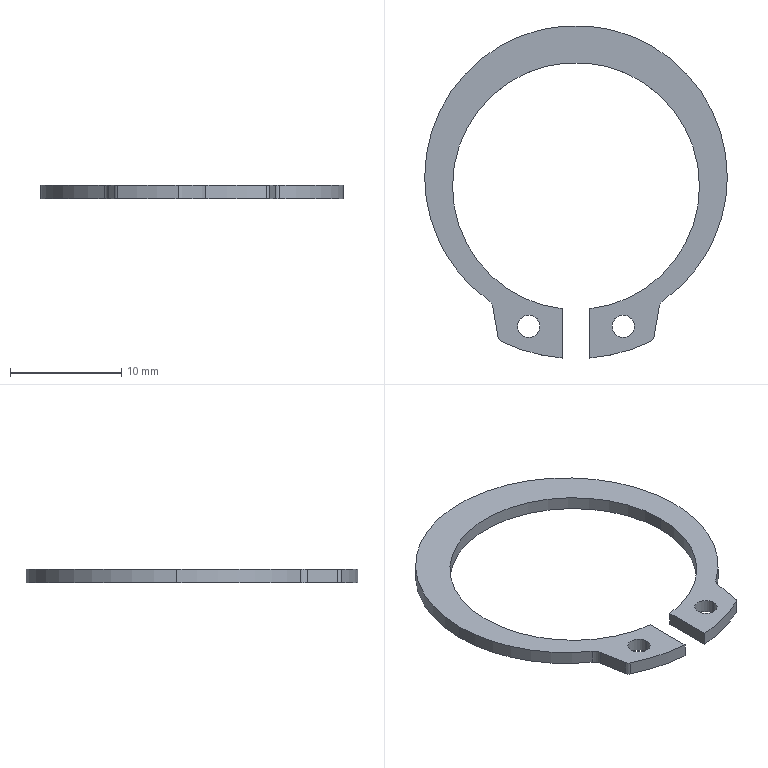Part | SolidWorks | features MoveCopyBody 1, Stock 1 | 1 solid | 22 faces | box 27.2 x 29.88 x 1.2 mm | volume 261.105 mm3 | cylinder 16 | plane 6 | commonest cylinder face diameters 2 x6 22.2 x3 27.2 x3 1 x2 31 x2
STEP:
#1=CARTESIAN_POINT('',(3.25,-12.603,-1.2));
#2=VERTEX_POINT('',#1);
#3=CARTESIAN_POINT('',(5.25,-12.603,-1.2));
#4=VERTEX_POINT('',#3);
#5=CARTESIAN_POINT('',(4.25,-12.603,-1.2));
#6=DIRECTION('',(0.,0.,1.));
#7=DIRECTION('',(-1.,0.,0.));
#8=AXIS2_PLACEMENT_3D('',#5,#6,#7);
#9=CIRCLE('',#8,1.);
#10=EDGE_CURVE('',#2,#4,#9,.T.);
#11=ORIENTED_EDGE('',*,*,#10,.F.);
#12=CARTESIAN_POINT('',(3.25,-12.603,0.));
#13=VERTEX_POINT('',#12);
#14=CARTESIAN_POINT('',(3.25,-12.603,-1.2));
#15=DIRECTION('',(0.,0.,1.));
#16=VECTOR('',#15,1000.);
#17=LINE('',#14,#16);
#18=EDGE_CURVE('',#2,#13,#17,.T.);
#19=ORIENTED_EDGE('',*,*,#18,.T.);
#20=CARTESIAN_POINT('',(5.25,-12.603,0.));
#21=VERTEX_POINT('',#20);
#22=CARTESIAN_POINT('',(4.25,-12.603,0.));
#23=DIRECTION('',(0.,0.,1.));
#24=DIRECTION('',(-1.,0.,0.));
#25=AXIS2_PLACEMENT_3D('',#22,#23,#24);
#26=CIRCLE('',#25,1.);
#27=EDGE_CURVE('',#13,#21,#26,.T.);
#28=ORIENTED_EDGE('',*,*,#27,.T.);
#29=CARTESIAN_POINT('',(5.25,-12.603,-1.2));
#30=DIRECTION('',(0.,0.,1.));
#31=VECTOR('',#30,1000.);
#32=LINE('',#29,#31);
#33=EDGE_CURVE('',#4,#21,#32,.T.);
#34=ORIENTED_EDGE('',*,*,#33,.F.);
#35=EDGE_LOOP('',(#11,#19,#28,#34));
#36=FACE_OUTER_BOUND('',#35,.T.);
#37=CARTESIAN_POINT('',(4.25,-12.603,-1.2));
#38=DIRECTION('',(0.,0.,1.));
#39=DIRECTION('',(1.,0.,0.));
#40=AXIS2_PLACEMENT_3D('',#37,#38,#39);
#41=CYLINDRICAL_SURFACE('',#40,1.);
#42=ADVANCED_FACE('',(#36),#41,.F.);
#43=CARTESIAN_POINT('',(-5.25,-12.603,-1.2));
#44=VERTEX_POINT('',#43);
#45=CARTESIAN_POINT('',(-3.25,-12.603,-1.2));
#46=VERTEX_POINT('',#45);
#47=CARTESIAN_POINT('',(-4.25,-12.603,-1.2));
#48=DIRECTION('',(0.,0.,1.));
#49=DIRECTION('',(1.,0.,0.));
#50=AXIS2_PLACEMENT_3D('',#47,#48,#49);
#51=CIRCLE('',#50,1.);
#52=EDGE_CURVE('',#44,#46,#51,.T.);
#53=ORIENTED_EDGE('',*,*,#52,.F.);
#54=CARTESIAN_POINT('',(-5.25,-12.603,0.));
#55=VERTEX_POINT('',#54);
#56=CARTESIAN_POINT('',(-5.25,-12.603,-1.2));
#57=DIRECTION('',(0.,0.,1.));
#58=VECTOR('',#57,1000.);
#59=LINE('',#56,#58);
#60=EDGE_CURVE('',#44,#55,#59,.T.);
#61=ORIENTED_EDGE('',*,*,#60,.T.);
#62=CARTESIAN_POINT('',(-3.25,-12.603,0.));
#63=VERTEX_POINT('',#62);
#64=CARTESIAN_POINT('',(-4.25,-12.603,0.));
#65=DIRECTION('',(0.,0.,1.));
#66=DIRECTION('',(1.,0.,0.));
#67=AXIS2_PLACEMENT_3D('',#64,#65,#66);
#68=CIRCLE('',#67,1.);
#69=EDGE_CURVE('',#55,#63,#68,.T.);
#70=ORIENTED_EDGE('',*,*,#69,.T.);
#71=CARTESIAN_POINT('',(-3.25,-12.603,-1.2));
#72=DIRECTION('',(0.,0.,1.));
#73=VECTOR('',#72,1000.);
#74=LINE('',#71,#73);
#75=EDGE_CURVE('',#46,#63,#74,.T.);
#76=ORIENTED_EDGE('',*,*,#75,.F.);
#77=EDGE_LOOP('',(#53,#61,#70,#76));
#78=FACE_OUTER_BOUND('',#77,.T.);
#79=CARTESIAN_POINT('',(-4.25,-12.603,-1.2));
#80=DIRECTION('',(0.,0.,1.));
#81=DIRECTION('',(1.,0.,0.));
#82=AXIS2_PLACEMENT_3D('',#79,#80,#81);
#83=CYLINDRICAL_SURFACE('',#82,1.);
#84=ADVANCED_FACE('',(#78),#83,.F.);
#85=CARTESIAN_POINT('',(13.6,0.83,-1.2));
#86=VERTEX_POINT('',#85);
#87=CARTESIAN_POINT('',(-13.6,0.83,-1.2));
#88=VERTEX_POINT('',#87);
#89=CARTESIAN_POINT('',(0.,0.83,-1.2));
#90=DIRECTION('',(0.,0.,1.));
#91=DIRECTION('',(1.,0.,0.));
#92=AXIS2_PLACEMENT_3D('',#89,#90,#91);
#93=CIRCLE('',#92,13.6);
#94=EDGE_CURVE('',#86,#88,#93,.T.);
#95=ORIENTED_EDGE('',*,*,#94,.T.);
#96=CARTESIAN_POINT('',(-13.6,0.83,0.));
#97=VERTEX_POINT('',#96);
#98=CARTESIAN_POINT('',(-13.6,0.83,-1.2));
#99=DIRECTION('',(0.,0.,1.));
#100=VECTOR('',#99,1000.);
#101=LINE('',#98,#100);
#102=EDGE_CURVE('',#88,#97,#101,.T.);
#103=ORIENTED_EDGE('',*,*,#102,.T.);
#104=CARTESIAN_POINT('',(13.6,0.83,0.));
#105=VERTEX_POINT('',#104);
#106=CARTESIAN_POINT('',(0.,0.83,0.));
#107=DIRECTION('',(0.,0.,1.));
#108=DIRECTION('',(1.,0.,0.));
#109=AXIS2_PLACEMENT_3D('',#106,#107,#108);
#110=CIRCLE('',#109,13.6);
#111=EDGE_CURVE('',#105,#97,#110,.T.);
#112=ORIENTED_EDGE('',*,*,#111,.F.);
#113=CARTESIAN_POINT('',(13.6,0.83,-1.2));
#114=DIRECTION('',(0.,0.,1.));
#115=VECTOR('',#114,1000.);
#116=LINE('',#113,#115);
#117=EDGE_CURVE('',#86,#105,#116,.T.);
#118=ORIENTED_EDGE('',*,*,#117,.F.);
#119=EDGE_LOOP('',(#95,#103,#112,#118));
#120=FACE_OUTER_BOUND('',#119,.T.);
#121=CARTESIAN_POINT('',(0.,0.83,-1.2));
#122=DIRECTION('',(0.,0.,1.));
#123=DIRECTION('',(1.,0.,0.));
#124=AXIS2_PLACEMENT_3D('',#121,#122,#123);
#125=CYLINDRICAL_SURFACE('',#124,13.6);
#126=ADVANCED_FACE('',(#120),#125,.T.);
#127=CARTESIAN_POINT('',(7.88,-10.255,-1.2));
#128=VERTEX_POINT('',#127);
#129=CARTESIAN_POINT('',(0.,0.83,-1.2));
#130=DIRECTION('',(0.,0.,1.));
#131=DIRECTION('',(1.,0.,0.));
#132=AXIS2_PLACEMENT_3D('',#129,#130,#131);
#133=CIRCLE('',#132,13.6);
#134=EDGE_CURVE('',#128,#86,#133,.T.);
#135=ORIENTED_EDGE('',*,*,#134,.T.);
#136=ORIENTED_EDGE('',*,*,#117,.T.);
#137=CARTESIAN_POINT('',(7.88,-10.255,0.));
#138=VERTEX_POINT('',#137);
#139=CARTESIAN_POINT('',(0.,0.83,0.));
#140=DIRECTION('',(0.,0.,1.));
#141=DIRECTION('',(1.,0.,0.));
#142=AXIS2_PLACEMENT_3D('',#139,#140,#141);
#143=CIRCLE('',#142,13.6);
#144=EDGE_CURVE('',#138,#105,#143,.T.);
#145=ORIENTED_EDGE('',*,*,#144,.F.);
#146=CARTESIAN_POINT('',(7.88,-10.255,-1.2));
#147=DIRECTION('',(0.,0.,-1.));
#148=VECTOR('',#147,1000.);
#149=LINE('',#146,#148);
#150=EDGE_CURVE('',#138,#128,#149,.T.);
#151=ORIENTED_EDGE('',*,*,#150,.T.);
#152=EDGE_LOOP('',(#135,#136,#145,#151));
#153=FACE_OUTER_BOUND('',#152,.T.);
#154=CARTESIAN_POINT('',(0.,0.83,-1.2));
#155=DIRECTION('',(0.,0.,1.));
#156=DIRECTION('',(1.,0.,0.));
#157=AXIS2_PLACEMENT_3D('',#154,#155,#156);
#158=CYLINDRICAL_SURFACE('',#157,13.6);
#159=ADVANCED_FACE('',(#153),#158,.T.);
#160=CARTESIAN_POINT('',(-1.25,-11.029,-1.2));
#161=VERTEX_POINT('',#160);
#162=CARTESIAN_POINT('',(-11.1,0.,-1.2));
#163=VERTEX_POINT('',#162);
#164=CARTESIAN_POINT('',(0.,0.,-1.2));
#165=DIRECTION('',(0.,0.,-1.));
#166=DIRECTION('',(1.,0.,0.));
#167=AXIS2_PLACEMENT_3D('',#164,#165,#166);
#168=CIRCLE('',#167,11.1);
#169=EDGE_CURVE('',#161,#163,#168,.T.);
#170=ORIENTED_EDGE('',*,*,#169,.T.);
#171=CARTESIAN_POINT('',(-11.1,0.,0.));
#172=VERTEX_POINT('',#171);
#173=CARTESIAN_POINT('',(-11.1,0.,-1.2));
#174=DIRECTION('',(0.,0.,1.));
#175=VECTOR('',#174,1000.);
#176=LINE('',#173,#175);
#177=EDGE_CURVE('',#163,#172,#176,.T.);
#178=ORIENTED_EDGE('',*,*,#177,.T.);
#179=CARTESIAN_POINT('',(-1.25,-11.029,0.));
#180=VERTEX_POINT('',#179);
#181=CARTESIAN_POINT('',(0.,0.,0.));
#182=DIRECTION('',(0.,0.,-1.));
#183=DIRECTION('',(1.,0.,0.));
#184=AXIS2_PLACEMENT_3D('',#181,#182,#183);
#185=CIRCLE('',#184,11.1);
#186=EDGE_CURVE('',#180,#172,#185,.T.);
#187=ORIENTED_EDGE('',*,*,#186,.F.);
#188=CARTESIAN_POINT('',(-1.25,-11.029,-1.2));
#189=DIRECTION('',(0.,0.,1.));
#190=VECTOR('',#189,1000.);
#191=LINE('',#188,#190);
#192=EDGE_CURVE('',#161,#180,#191,.T.);
#193=ORIENTED_EDGE('',*,*,#192,.F.);
#194=EDGE_LOOP('',(#170,#178,#187,#193));
#195=FACE_OUTER_BOUND('',#194,.T.);
#196=CARTESIAN_POINT('',(0.,0.,-1.2));
#197=DIRECTION('',(0.,0.,1.));
#198=DIRECTION('',(1.,0.,0.));
#199=AXIS2_PLACEMENT_3D('',#196,#197,#198);
#200=CYLINDRICAL_SURFACE('',#199,11.1);
#201=ADVANCED_FACE('',(#195),#200,.F.);
#202=ORIENTED_EDGE('',*,*,#177,.F.);
#203=CARTESIAN_POINT('',(11.1,0.,-1.2));
#204=VERTEX_POINT('',#203);
#205=CARTESIAN_POINT('',(0.,0.,-1.2));
#206=DIRECTION('',(0.,0.,-1.));
#207=DIRECTION('',(1.,0.,0.));
#208=AXIS2_PLACEMENT_3D('',#205,#206,#207);
#209=CIRCLE('',#208,11.1);
#210=EDGE_CURVE('',#163,#204,#209,.T.);
#211=ORIENTED_EDGE('',*,*,#210,.T.);
#212=CARTESIAN_POINT('',(11.1,0.,0.));
#213=VERTEX_POINT('',#212);
#214=CARTESIAN_POINT('',(11.1,0.,-1.2));
#215=DIRECTION('',(0.,0.,1.));
#216=VECTOR('',#215,1000.);
#217=LINE('',#214,#216);
#218=EDGE_CURVE('',#204,#213,#217,.T.);
#219=ORIENTED_EDGE('',*,*,#218,.T.);
#220=CARTESIAN_POINT('',(0.,0.,0.));
#221=DIRECTION('',(0.,0.,-1.));
#222=DIRECTION('',(1.,0.,0.));
#223=AXIS2_PLACEMENT_3D('',#220,#221,#222);
#224=CIRCLE('',#223,11.1);
#225=EDGE_CURVE('',#172,#213,#224,.T.);
#226=ORIENTED_EDGE('',*,*,#225,.F.);
#227=EDGE_LOOP('',(#202,#211,#219,#226));
#228=FACE_OUTER_BOUND('',#227,.T.);
#229=CARTESIAN_POINT('',(0.,0.,-1.2));
#230=DIRECTION('',(0.,0.,1.));
#231=DIRECTION('',(1.,0.,0.));
#232=AXIS2_PLACEMENT_3D('',#229,#230,#231);
#233=CYLINDRICAL_SURFACE('',#232,11.1);
#234=ADVANCED_FACE('',(#228),#233,.F.);
#235=CARTESIAN_POINT('',(1.25,-15.45,-1.2));
#236=VERTEX_POINT('',#235);
#237=CARTESIAN_POINT('',(6.721,-13.967,-1.2));
#238=VERTEX_POINT('',#237);
#239=CARTESIAN_POINT('',(0.,0.,-1.2));
#240=DIRECTION('',(0.,0.,1.));
#241=DIRECTION('',(-1.,0.,0.));
#242=AXIS2_PLACEMENT_3D('',#239,#240,#241);
#243=CIRCLE('',#242,15.5);
#244=EDGE_CURVE('',#236,#238,#243,.T.);
#245=ORIENTED_EDGE('',*,*,#244,.T.);
#246=CARTESIAN_POINT('',(6.721,-13.967,0.));
#247=VERTEX_POINT('',#246);
#248=CARTESIAN_POINT('',(6.721,-13.967,-1.2));
#249=DIRECTION('',(0.,0.,1.));
#250=VECTOR('',#249,1000.);
#251=LINE('',#248,#250);
#252=EDGE_CURVE('',#238,#247,#251,.T.);
#253=ORIENTED_EDGE('',*,*,#252,.T.);
#254=CARTESIAN_POINT('',(1.25,-15.45,0.));
#255=VERTEX_POINT('',#254);
#256=CARTESIAN_POINT('',(0.,0.,0.));
#257=DIRECTION('',(0.,0.,1.));
#258=DIRECTION('',(-1.,0.,0.));
#259=AXIS2_PLACEMENT_3D('',#256,#257,#258);
#260=CIRCLE('',#259,15.5);
#261=EDGE_CURVE('',#255,#247,#260,.T.);
#262=ORIENTED_EDGE('',*,*,#261,.F.);
#263=CARTESIAN_POINT('',(1.25,-15.45,-1.2));
#264=DIRECTION('',(0.,0.,1.));
#265=VECTOR('',#264,1000.);
#266=LINE('',#263,#265);
#267=EDGE_CURVE('',#236,#255,#266,.T.);
#268=ORIENTED_EDGE('',*,*,#267,.F.);
#269=EDGE_LOOP('',(#245,#253,#262,#268));
#270=FACE_OUTER_BOUND('',#269,.T.);
#271=CARTESIAN_POINT('',(0.,0.,-1.2));
#272=DIRECTION('',(0.,0.,1.));
#273=DIRECTION('',(1.,0.,0.));
#274=AXIS2_PLACEMENT_3D('',#271,#272,#273);
#275=CYLINDRICAL_SURFACE('',#274,15.5);
#276=ADVANCED_FACE('',(#270),#275,.T.);
#277=CARTESIAN_POINT('',(1.25,-11.029,0.));
#278=VERTEX_POINT('',#277);
#279=CARTESIAN_POINT('',(1.25,-11.029,0.));
#280=DIRECTION('',(0.,-1.,0.));
#281=VECTOR('',#280,1000.);
#282=LINE('',#279,#281);
#283=EDGE_CURVE('',#278,#255,#282,.T.);
#284=ORIENTED_EDGE('',*,*,#283,.F.);
#285=CARTESIAN_POINT('',(1.25,-11.029,-1.2));
#286=VERTEX_POINT('',#285);
#287=CARTESIAN_POINT('',(1.25,-11.029,-1.2));
#288=DIRECTION('',(0.,0.,1.));
#289=VECTOR('',#288,1000.);
#290=LINE('',#287,#289);
#291=EDGE_CURVE('',#286,#278,#290,.T.);
#292=ORIENTED_EDGE('',*,*,#291,.F.);
#293=CARTESIAN_POINT('',(1.25,-11.029,-1.2));
#294=DIRECTION('',(0.,-1.,0.));
#295=VECTOR('',#294,1000.);
#296=LINE('',#293,#295);
#297=EDGE_CURVE('',#286,#236,#296,.T.);
#298=ORIENTED_EDGE('',*,*,#297,.T.);
#299=ORIENTED_EDGE('',*,*,#267,.T.);
#300=EDGE_LOOP('',(#284,#292,#298,#299));
#301=FACE_OUTER_BOUND('',#300,.T.);
#302=CARTESIAN_POINT('',(1.25,-11.029,-1.2));
#303=DIRECTION('',(-1.,0.,0.));
#304=DIRECTION('',(0.,-1.,0.));
#305=AXIS2_PLACEMENT_3D('',#302,#303,#304);
#306=PLANE('',#305);
#307=ADVANCED_FACE('',(#301),#306,.T.);
#308=ORIENTED_EDGE('',*,*,#218,.F.);
#309=CARTESIAN_POINT('',(0.,0.,-1.2));
#310=DIRECTION('',(0.,0.,-1.));
#311=DIRECTION('',(1.,0.,0.));
#312=AXIS2_PLACEMENT_3D('',#309,#310,#311);
#313=CIRCLE('',#312,11.1);
#314=EDGE_CURVE('',#204,#286,#313,.T.);
#315=ORIENTED_EDGE('',*,*,#314,.T.);
#316=ORIENTED_EDGE('',*,*,#291,.T.);
#317=CARTESIAN_POINT('',(0.,0.,0.));
#318=DIRECTION('',(0.,0.,-1.));
#319=DIRECTION('',(1.,0.,0.));
#320=AXIS2_PLACEMENT_3D('',#317,#318,#319);
#321=CIRCLE('',#320,11.1);
#322=EDGE_CURVE('',#213,#278,#321,.T.);
#323=ORIENTED_EDGE('',*,*,#322,.F.);
#324=EDGE_LOOP('',(#308,#315,#316,#323));
#325=FACE_OUTER_BOUND('',#324,.T.);
#326=CARTESIAN_POINT('',(0.,0.,-1.2));
#327=DIRECTION('',(0.,0.,1.));
#328=DIRECTION('',(1.,0.,0.));
#329=AXIS2_PLACEMENT_3D('',#326,#327,#328);
#330=CYLINDRICAL_SURFACE('',#329,11.1);
#331=ADVANCED_FACE('',(#325),#330,.F.);
#332=CARTESIAN_POINT('',(-1.25,-15.45,0.));
#333=VERTEX_POINT('',#332);
#334=CARTESIAN_POINT('',(-1.25,-11.029,0.));
#335=DIRECTION('',(0.,1.,0.));
#336=VECTOR('',#335,1000.);
#337=LINE('',#334,#336);
#338=EDGE_CURVE('',#333,#180,#337,.T.);
#339=ORIENTED_EDGE('',*,*,#338,.F.);
#340=CARTESIAN_POINT('',(-1.25,-15.45,-1.2));
#341=VERTEX_POINT('',#340);
#342=CARTESIAN_POINT('',(-1.25,-15.45,-1.2));
#343=DIRECTION('',(0.,0.,1.));
#344=VECTOR('',#343,1000.);
#345=LINE('',#342,#344);
#346=EDGE_CURVE('',#341,#333,#345,.T.);
#347=ORIENTED_EDGE('',*,*,#346,.F.);
#348=CARTESIAN_POINT('',(-1.25,-11.029,-1.2));
#349=DIRECTION('',(0.,1.,0.));
#350=VECTOR('',#349,1000.);
#351=LINE('',#348,#350);
#352=EDGE_CURVE('',#341,#161,#351,.T.);
#353=ORIENTED_EDGE('',*,*,#352,.T.);
#354=ORIENTED_EDGE('',*,*,#192,.T.);
#355=EDGE_LOOP('',(#339,#347,#353,#354));
#356=FACE_OUTER_BOUND('',#355,.T.);
#357=CARTESIAN_POINT('',(-1.25,-11.029,-1.2));
#358=DIRECTION('',(1.,0.,0.));
#359=DIRECTION('',(0.,1.,0.));
#360=AXIS2_PLACEMENT_3D('',#357,#358,#359);
#361=PLANE('',#360);
#362=ADVANCED_FACE('',(#356),#361,.T.);
#363=CARTESIAN_POINT('',(-6.721,-13.967,0.));
#364=VERTEX_POINT('',#363);
#365=CARTESIAN_POINT('',(0.,0.,0.));
#366=DIRECTION('',(0.,0.,1.));
#367=DIRECTION('',(1.,0.,0.));
#368=AXIS2_PLACEMENT_3D('',#365,#366,#367);
#369=CIRCLE('',#368,15.5);
#370=EDGE_CURVE('',#364,#333,#369,.T.);
#371=ORIENTED_EDGE('',*,*,#370,.F.);
#372=CARTESIAN_POINT('',(-6.721,-13.967,-1.2));
#373=VERTEX_POINT('',#372);
#374=CARTESIAN_POINT('',(-6.721,-13.967,-1.2));
#375=DIRECTION('',(0.,0.,-1.));
#376=VECTOR('',#375,1000.);
#377=LINE('',#374,#376);
#378=EDGE_CURVE('',#364,#373,#377,.T.);
#379=ORIENTED_EDGE('',*,*,#378,.T.);
#380=CARTESIAN_POINT('',(0.,0.,-1.2));
#381=DIRECTION('',(0.,0.,1.));
#382=DIRECTION('',(1.,0.,0.));
#383=AXIS2_PLACEMENT_3D('',#380,#381,#382);
#384=CIRCLE('',#383,15.5);
#385=EDGE_CURVE('',#373,#341,#384,.T.);
#386=ORIENTED_EDGE('',*,*,#385,.T.);
#387=ORIENTED_EDGE('',*,*,#346,.T.);
#388=EDGE_LOOP('',(#371,#379,#386,#387));
#389=FACE_OUTER_BOUND('',#388,.T.);
#390=CARTESIAN_POINT('',(0.,0.,-1.2));
#391=DIRECTION('',(0.,0.,1.));
#392=DIRECTION('',(1.,0.,0.));
#393=AXIS2_PLACEMENT_3D('',#390,#391,#392);
#394=CYLINDRICAL_SURFACE('',#393,15.5);
#395=ADVANCED_FACE('',(#389),#394,.T.);
#396=CARTESIAN_POINT('',(-7.474,-10.896,0.));
#397=VERTEX_POINT('',#396);
#398=CARTESIAN_POINT('',(-6.997,-13.603,0.));
#399=VERTEX_POINT('',#398);
#400=CARTESIAN_POINT('',(-7.547,-10.484,0.));
#401=DIRECTION('',(0.1736,-0.9848,0.));
#402=VECTOR('',#401,1000.);
#403=LINE('',#400,#402);
#404=EDGE_CURVE('',#397,#399,#403,.T.);
#405=ORIENTED_EDGE('',*,*,#404,.F.);
#406=CARTESIAN_POINT('',(-7.474,-10.896,-1.2));
#407=VERTEX_POINT('',#406);
#408=CARTESIAN_POINT('',(-7.474,-10.896,-1.2));
#409=DIRECTION('',(0.,0.,-1.));
#410=VECTOR('',#409,1000.);
#411=LINE('',#408,#410);
#412=EDGE_CURVE('',#397,#407,#411,.T.);
#413=ORIENTED_EDGE('',*,*,#412,.T.);
#414=CARTESIAN_POINT('',(-6.997,-13.603,-1.2));
#415=VERTEX_POINT('',#414);
#416=CARTESIAN_POINT('',(-7.547,-10.484,-1.2));
#417=DIRECTION('',(0.1736,-0.9848,0.));
#418=VECTOR('',#417,1000.);
#419=LINE('',#416,#418);
#420=EDGE_CURVE('',#407,#415,#419,.T.);
#421=ORIENTED_EDGE('',*,*,#420,.T.);
#422=CARTESIAN_POINT('',(-6.997,-13.603,-1.2));
#423=DIRECTION('',(0.,0.,1.));
#424=VECTOR('',#423,1000.);
#425=LINE('',#422,#424);
#426=EDGE_CURVE('',#415,#399,#425,.T.);
#427=ORIENTED_EDGE('',*,*,#426,.T.);
#428=EDGE_LOOP('',(#405,#413,#421,#427));
#429=FACE_OUTER_BOUND('',#428,.T.);
#430=CARTESIAN_POINT('',(-7.547,-10.484,-1.2));
#431=DIRECTION('',(-0.9848,-0.1736,0.));
#432=DIRECTION('',(0.1736,-0.9848,0.));
#433=AXIS2_PLACEMENT_3D('',#430,#431,#432);
#434=PLANE('',#433);
#435=ADVANCED_FACE('',(#429),#434,.T.);
#436=ORIENTED_EDGE('',*,*,#102,.F.);
#437=CARTESIAN_POINT('',(-7.88,-10.255,-1.2));
#438=VERTEX_POINT('',#437);
#439=CARTESIAN_POINT('',(0.,0.83,-1.2));
#440=DIRECTION('',(0.,0.,1.));
#441=DIRECTION('',(1.,0.,0.));
#442=AXIS2_PLACEMENT_3D('',#439,#440,#441);
#443=CIRCLE('',#442,13.6);
#444=EDGE_CURVE('',#88,#438,#443,.T.);
#445=ORIENTED_EDGE('',*,*,#444,.T.);
#446=CARTESIAN_POINT('',(-7.88,-10.255,0.));
#447=VERTEX_POINT('',#446);
#448=CARTESIAN_POINT('',(-7.88,-10.255,-1.2));
#449=DIRECTION('',(0.,0.,1.));
#450=VECTOR('',#449,1000.);
#451=LINE('',#448,#450);
#452=EDGE_CURVE('',#438,#447,#451,.T.);
#453=ORIENTED_EDGE('',*,*,#452,.T.);
#454=CARTESIAN_POINT('',(0.,0.83,0.));
#455=DIRECTION('',(0.,0.,1.));
#456=DIRECTION('',(1.,0.,0.));
#457=AXIS2_PLACEMENT_3D('',#454,#455,#456);
#458=CIRCLE('',#457,13.6);
#459=EDGE_CURVE('',#97,#447,#458,.T.);
#460=ORIENTED_EDGE('',*,*,#459,.F.);
#461=EDGE_LOOP('',(#436,#445,#453,#460));
#462=FACE_OUTER_BOUND('',#461,.T.);
#463=CARTESIAN_POINT('',(0.,0.83,-1.2));
#464=DIRECTION('',(0.,0.,1.));
#465=DIRECTION('',(1.,0.,0.));
#466=AXIS2_PLACEMENT_3D('',#463,#464,#465);
#467=CYLINDRICAL_SURFACE('',#466,13.6);
#468=ADVANCED_FACE('',(#462),#467,.T.);
#469=CARTESIAN_POINT('',(6.997,-13.603,-1.2));
#470=VERTEX_POINT('',#469);
#471=CARTESIAN_POINT('',(7.474,-10.896,-1.2));
#472=VERTEX_POINT('',#471);
#473=CARTESIAN_POINT('',(7.547,-10.484,-1.2));
#474=DIRECTION('',(0.1736,0.9848,0.));
#475=VECTOR('',#474,1000.);
#476=LINE('',#473,#475);
#477=EDGE_CURVE('',#470,#472,#476,.T.);
#478=ORIENTED_EDGE('',*,*,#477,.T.);
#479=CARTESIAN_POINT('',(7.474,-10.896,0.));
#480=VERTEX_POINT('',#479);
#481=CARTESIAN_POINT('',(7.474,-10.896,0.));
#482=DIRECTION('',(0.,0.,1.));
#483=VECTOR('',#482,1000.);
#484=LINE('',#481,#483);
#485=EDGE_CURVE('',#472,#480,#484,.T.);
#486=ORIENTED_EDGE('',*,*,#485,.T.);
#487=CARTESIAN_POINT('',(6.997,-13.603,0.));
#488=VERTEX_POINT('',#487);
#489=CARTESIAN_POINT('',(7.547,-10.484,0.));
#490=DIRECTION('',(0.1736,0.9848,0.));
#491=VECTOR('',#490,1000.);
#492=LINE('',#489,#491);
#493=EDGE_CURVE('',#488,#480,#492,.T.);
#494=ORIENTED_EDGE('',*,*,#493,.F.);
#495=CARTESIAN_POINT('',(6.997,-13.603,-1.2));
#496=DIRECTION('',(0.,0.,-1.));
#497=VECTOR('',#496,1000.);
#498=LINE('',#495,#497);
#499=EDGE_CURVE('',#488,#470,#498,.T.);
#500=ORIENTED_EDGE('',*,*,#499,.T.);
#501=EDGE_LOOP('',(#478,#486,#494,#500));
#502=FACE_OUTER_BOUND('',#501,.T.);
#503=CARTESIAN_POINT('',(7.547,-10.484,-1.2));
#504=DIRECTION('',(0.9848,-0.1736,0.));
#505=DIRECTION('',(0.1736,0.9848,0.));
#506=AXIS2_PLACEMENT_3D('',#503,#504,#505);
#507=PLANE('',#506);
#508=ADVANCED_FACE('',(#502),#507,.T.);
#509=CARTESIAN_POINT('',(4.25,-12.603,-1.2));
#510=DIRECTION('',(0.,0.,1.));
#511=DIRECTION('',(-1.,0.,0.));
#512=AXIS2_PLACEMENT_3D('',#509,#510,#511);
#513=CIRCLE('',#512,1.);
#514=EDGE_CURVE('',#4,#2,#513,.T.);
#515=ORIENTED_EDGE('',*,*,#514,.T.);
#516=ORIENTED_EDGE('',*,*,#10,.T.);
#517=EDGE_LOOP('',(#515,#516));
#518=FACE_BOUND('',#517,.T.);
#519=CARTESIAN_POINT('',(-4.25,-12.603,-1.2));
#520=DIRECTION('',(0.,0.,1.));
#521=DIRECTION('',(1.,0.,0.));
#522=AXIS2_PLACEMENT_3D('',#519,#520,#521);
#523=CIRCLE('',#522,1.);
#524=EDGE_CURVE('',#46,#44,#523,.T.);
#525=ORIENTED_EDGE('',*,*,#524,.T.);
#526=ORIENTED_EDGE('',*,*,#52,.T.);
#527=EDGE_LOOP('',(#525,#526));
#528=FACE_BOUND('',#527,.T.);
#529=ORIENTED_EDGE('',*,*,#385,.F.);
#530=CARTESIAN_POINT('',(-6.505,-13.516,-1.2));
#531=DIRECTION('',(0.,0.,-1.));
#532=DIRECTION('',(-1.,0.,0.));
#533=AXIS2_PLACEMENT_3D('',#530,#531,#532);
#534=CIRCLE('',#533,0.5);
#535=EDGE_CURVE('',#373,#415,#534,.T.);
#536=ORIENTED_EDGE('',*,*,#535,.T.);
#537=ORIENTED_EDGE('',*,*,#420,.F.);
#538=CARTESIAN_POINT('',(-8.459,-11.07,-1.2));
#539=DIRECTION('',(0.,0.,1.));
#540=DIRECTION('',(-1.,0.,0.));
#541=AXIS2_PLACEMENT_3D('',#538,#539,#540);
#542=CIRCLE('',#541,1.);
#543=EDGE_CURVE('',#407,#438,#542,.T.);
#544=ORIENTED_EDGE('',*,*,#543,.T.);
#545=ORIENTED_EDGE('',*,*,#444,.F.);
#546=ORIENTED_EDGE('',*,*,#94,.F.);
#547=ORIENTED_EDGE('',*,*,#134,.F.);
#548=CARTESIAN_POINT('',(8.459,-11.07,-1.2));
#549=DIRECTION('',(0.,0.,1.));
#550=DIRECTION('',(-1.,0.,0.));
#551=AXIS2_PLACEMENT_3D('',#548,#549,#550);
#552=CIRCLE('',#551,1.);
#553=EDGE_CURVE('',#128,#472,#552,.T.);
#554=ORIENTED_EDGE('',*,*,#553,.T.);
#555=ORIENTED_EDGE('',*,*,#477,.F.);
#556=CARTESIAN_POINT('',(6.505,-13.516,-1.2));
#557=DIRECTION('',(0.,0.,-1.));
#558=DIRECTION('',(-1.,0.,0.));
#559=AXIS2_PLACEMENT_3D('',#556,#557,#558);
#560=CIRCLE('',#559,0.5);
#561=EDGE_CURVE('',#470,#238,#560,.T.);
#562=ORIENTED_EDGE('',*,*,#561,.T.);
#563=ORIENTED_EDGE('',*,*,#244,.F.);
#564=ORIENTED_EDGE('',*,*,#297,.F.);
#565=ORIENTED_EDGE('',*,*,#314,.F.);
#566=ORIENTED_EDGE('',*,*,#210,.F.);
#567=ORIENTED_EDGE('',*,*,#169,.F.);
#568=ORIENTED_EDGE('',*,*,#352,.F.);
#569=EDGE_LOOP('',(#529,#536,#537,#544,#545,#546,#547,#554,#555,#562,#563,#564,#565,#566,#567,#568));
#570=FACE_OUTER_BOUND('',#569,.T.);
#571=CARTESIAN_POINT('',(0.,0.,-1.2));
#572=DIRECTION('',(0.,0.,-1.));
#573=DIRECTION('',(-1.,0.,0.));
#574=AXIS2_PLACEMENT_3D('',#571,#572,#573);
#575=PLANE('',#574);
#576=ADVANCED_FACE('',(#518,#528,#570),#575,.T.);
#577=CARTESIAN_POINT('',(4.25,-12.603,0.));
#578=DIRECTION('',(0.,0.,1.));
#579=DIRECTION('',(-1.,0.,0.));
#580=AXIS2_PLACEMENT_3D('',#577,#578,#579);
#581=CIRCLE('',#580,1.);
#582=EDGE_CURVE('',#21,#13,#581,.T.);
#583=ORIENTED_EDGE('',*,*,#582,.F.);
#584=ORIENTED_EDGE('',*,*,#27,.F.);
#585=EDGE_LOOP('',(#583,#584));
#586=FACE_BOUND('',#585,.T.);
#587=CARTESIAN_POINT('',(-4.25,-12.603,0.));
#588=DIRECTION('',(0.,0.,1.));
#589=DIRECTION('',(1.,0.,0.));
#590=AXIS2_PLACEMENT_3D('',#587,#588,#589);
#591=CIRCLE('',#590,1.);
#592=EDGE_CURVE('',#63,#55,#591,.T.);
#593=ORIENTED_EDGE('',*,*,#592,.F.);
#594=ORIENTED_EDGE('',*,*,#69,.F.);
#595=EDGE_LOOP('',(#593,#594));
#596=FACE_BOUND('',#595,.T.);
#597=ORIENTED_EDGE('',*,*,#144,.T.);
#598=ORIENTED_EDGE('',*,*,#111,.T.);
#599=ORIENTED_EDGE('',*,*,#459,.T.);
#600=CARTESIAN_POINT('',(-8.459,-11.07,0.));
#601=DIRECTION('',(0.,0.,-1.));
#602=DIRECTION('',(-1.,0.,0.));
#603=AXIS2_PLACEMENT_3D('',#600,#601,#602);
#604=CIRCLE('',#603,1.);
#605=EDGE_CURVE('',#447,#397,#604,.T.);
#606=ORIENTED_EDGE('',*,*,#605,.T.);
#607=ORIENTED_EDGE('',*,*,#404,.T.);
#608=CARTESIAN_POINT('',(-6.505,-13.516,0.));
#609=DIRECTION('',(0.,0.,1.));
#610=DIRECTION('',(-1.,0.,0.));
#611=AXIS2_PLACEMENT_3D('',#608,#609,#610);
#612=CIRCLE('',#611,0.5);
#613=EDGE_CURVE('',#399,#364,#612,.T.);
#614=ORIENTED_EDGE('',*,*,#613,.T.);
#615=ORIENTED_EDGE('',*,*,#370,.T.);
#616=ORIENTED_EDGE('',*,*,#338,.T.);
#617=ORIENTED_EDGE('',*,*,#186,.T.);
#618=ORIENTED_EDGE('',*,*,#225,.T.);
#619=ORIENTED_EDGE('',*,*,#322,.T.);
#620=ORIENTED_EDGE('',*,*,#283,.T.);
#621=ORIENTED_EDGE('',*,*,#261,.T.);
#622=CARTESIAN_POINT('',(6.505,-13.516,0.));
#623=DIRECTION('',(0.,0.,1.));
#624=DIRECTION('',(-1.,0.,0.));
#625=AXIS2_PLACEMENT_3D('',#622,#623,#624);
#626=CIRCLE('',#625,0.5);
#627=EDGE_CURVE('',#247,#488,#626,.T.);
#628=ORIENTED_EDGE('',*,*,#627,.T.);
#629=ORIENTED_EDGE('',*,*,#493,.T.);
#630=CARTESIAN_POINT('',(8.459,-11.07,0.));
#631=DIRECTION('',(0.,0.,-1.));
#632=DIRECTION('',(-1.,0.,0.));
#633=AXIS2_PLACEMENT_3D('',#630,#631,#632);
#634=CIRCLE('',#633,1.);
#635=EDGE_CURVE('',#480,#138,#634,.T.);
#636=ORIENTED_EDGE('',*,*,#635,.T.);
#637=EDGE_LOOP('',(#597,#598,#599,#606,#607,#614,#615,#616,#617,#618,#619,#620,#621,#628,#629,#636));
#638=FACE_OUTER_BOUND('',#637,.T.);
#639=CARTESIAN_POINT('',(0.,0.,0.));
#640=DIRECTION('',(0.,0.,-1.));
#641=DIRECTION('',(-1.,0.,0.));
#642=AXIS2_PLACEMENT_3D('',#639,#640,#641);
#643=PLANE('',#642);
#644=ADVANCED_FACE('',(#586,#596,#638),#643,.F.);
#645=ORIENTED_EDGE('',*,*,#60,.F.);
#646=ORIENTED_EDGE('',*,*,#524,.F.);
#647=ORIENTED_EDGE('',*,*,#75,.T.);
#648=ORIENTED_EDGE('',*,*,#592,.T.);
#649=EDGE_LOOP('',(#645,#646,#647,#648));
#650=FACE_OUTER_BOUND('',#649,.T.);
#651=CARTESIAN_POINT('',(-4.25,-12.603,-1.2));
#652=DIRECTION('',(0.,0.,1.));
#653=DIRECTION('',(1.,0.,0.));
#654=AXIS2_PLACEMENT_3D('',#651,#652,#653);
#655=CYLINDRICAL_SURFACE('',#654,1.);
#656=ADVANCED_FACE('',(#650),#655,.F.);
#657=ORIENTED_EDGE('',*,*,#18,.F.);
#658=ORIENTED_EDGE('',*,*,#514,.F.);
#659=ORIENTED_EDGE('',*,*,#33,.T.);
#660=ORIENTED_EDGE('',*,*,#582,.T.);
#661=EDGE_LOOP('',(#657,#658,#659,#660));
#662=FACE_OUTER_BOUND('',#661,.T.);
#663=CARTESIAN_POINT('',(4.25,-12.603,-1.2));
#664=DIRECTION('',(0.,0.,1.));
#665=DIRECTION('',(1.,0.,0.));
#666=AXIS2_PLACEMENT_3D('',#663,#664,#665);
#667=CYLINDRICAL_SURFACE('',#666,1.);
#668=ADVANCED_FACE('',(#662),#667,.F.);
#669=ORIENTED_EDGE('',*,*,#535,.F.);
#670=ORIENTED_EDGE('',*,*,#378,.F.);
#671=ORIENTED_EDGE('',*,*,#613,.F.);
#672=ORIENTED_EDGE('',*,*,#426,.F.);
#673=EDGE_LOOP('',(#669,#670,#671,#672));
#674=FACE_OUTER_BOUND('',#673,.T.);
#675=CARTESIAN_POINT('',(-6.505,-13.516,-1.2));
#676=DIRECTION('',(0.,0.,1.));
#677=DIRECTION('',(1.,0.,0.));
#678=AXIS2_PLACEMENT_3D('',#675,#676,#677);
#679=CYLINDRICAL_SURFACE('',#678,0.5);
#680=ADVANCED_FACE('',(#674),#679,.T.);
#681=ORIENTED_EDGE('',*,*,#561,.F.);
#682=ORIENTED_EDGE('',*,*,#499,.F.);
#683=ORIENTED_EDGE('',*,*,#627,.F.);
#684=ORIENTED_EDGE('',*,*,#252,.F.);
#685=EDGE_LOOP('',(#681,#682,#683,#684));
#686=FACE_OUTER_BOUND('',#685,.T.);
#687=CARTESIAN_POINT('',(6.505,-13.516,-1.2));
#688=DIRECTION('',(0.,0.,1.));
#689=DIRECTION('',(1.,0.,0.));
#690=AXIS2_PLACEMENT_3D('',#687,#688,#689);
#691=CYLINDRICAL_SURFACE('',#690,0.5);
#692=ADVANCED_FACE('',(#686),#691,.T.);
#693=ORIENTED_EDGE('',*,*,#553,.F.);
#694=ORIENTED_EDGE('',*,*,#150,.F.);
#695=ORIENTED_EDGE('',*,*,#635,.F.);
#696=ORIENTED_EDGE('',*,*,#485,.F.);
#697=EDGE_LOOP('',(#693,#694,#695,#696));
#698=FACE_OUTER_BOUND('',#697,.T.);
#699=CARTESIAN_POINT('',(8.459,-11.07,-1.2));
#700=DIRECTION('',(0.,0.,1.));
#701=DIRECTION('',(1.,0.,0.));
#702=AXIS2_PLACEMENT_3D('',#699,#700,#701);
#703=CYLINDRICAL_SURFACE('',#702,1.);
#704=ADVANCED_FACE('',(#698),#703,.F.);
#705=ORIENTED_EDGE('',*,*,#543,.F.);
#706=ORIENTED_EDGE('',*,*,#412,.F.);
#707=ORIENTED_EDGE('',*,*,#605,.F.);
#708=ORIENTED_EDGE('',*,*,#452,.F.);
#709=EDGE_LOOP('',(#705,#706,#707,#708));
#710=FACE_OUTER_BOUND('',#709,.T.);
#711=CARTESIAN_POINT('',(-8.459,-11.07,-1.2));
#712=DIRECTION('',(0.,0.,1.));
#713=DIRECTION('',(1.,0.,0.));
#714=AXIS2_PLACEMENT_3D('',#711,#712,#713);
#715=CYLINDRICAL_SURFACE('',#714,1.);
#716=ADVANCED_FACE('',(#710),#715,.F.);
#717=CLOSED_SHELL('',(#42,#84,#126,#159,#201,#234,#276,#307,#331,#362,#395,#435,#468,#508,#576,#644,#656,#668,#680,#692,#704,#716));
#718=MANIFOLD_SOLID_BREP('',#717);
#719=CARTESIAN_POINT('',(0.,0.,0.));
#720=DIRECTION('',(0.,0.,1.));
#721=DIRECTION('',(1.,0.,0.));
#722=AXIS2_PLACEMENT_3D('',#719,#720,#721);
#723=(LENGTH_UNIT()NAMED_UNIT(*)SI_UNIT(.MILLI.,.METRE.));
#724=UNCERTAINTY_MEASURE_WITH_UNIT(LENGTH_MEASURE(0.00001),#723,'','');
#725=(NAMED_UNIT(*)PLANE_ANGLE_UNIT()SI_UNIT($,.RADIAN.));
#726=(NAMED_UNIT(*)SI_UNIT($,.STERADIAN.)SOLID_ANGLE_UNIT());
#727=(GEOMETRIC_REPRESENTATION_CONTEXT(3)GLOBAL_UNCERTAINTY_ASSIGNED_CONTEXT((#724))GLOBAL_UNIT_ASSIGNED_CONTEXT((#723,#725,#726))REPRESENTATION_CONTEXT('',''));
#728=ADVANCED_BREP_SHAPE_REPRESENTATION('',(#718,#722),#727);